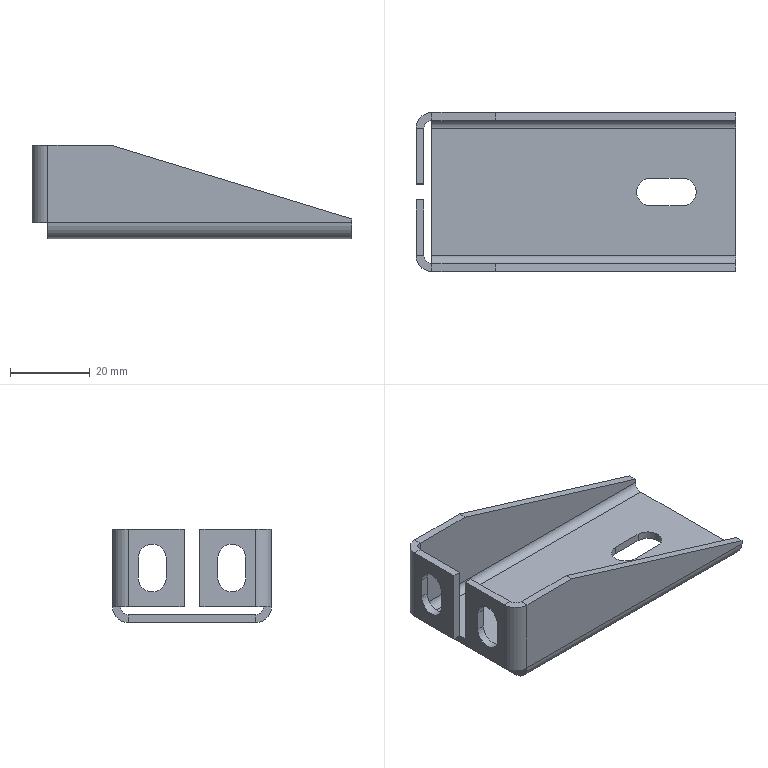Part | STEP file | 64644335 | 1 solid | 52 faces | box 80.5 x 40 x 23.5 mm | volume 11043 mm3 | plane 38 | cylinder 14 | commonest cylinder face diameters 7 x6 4 x4 8 x4